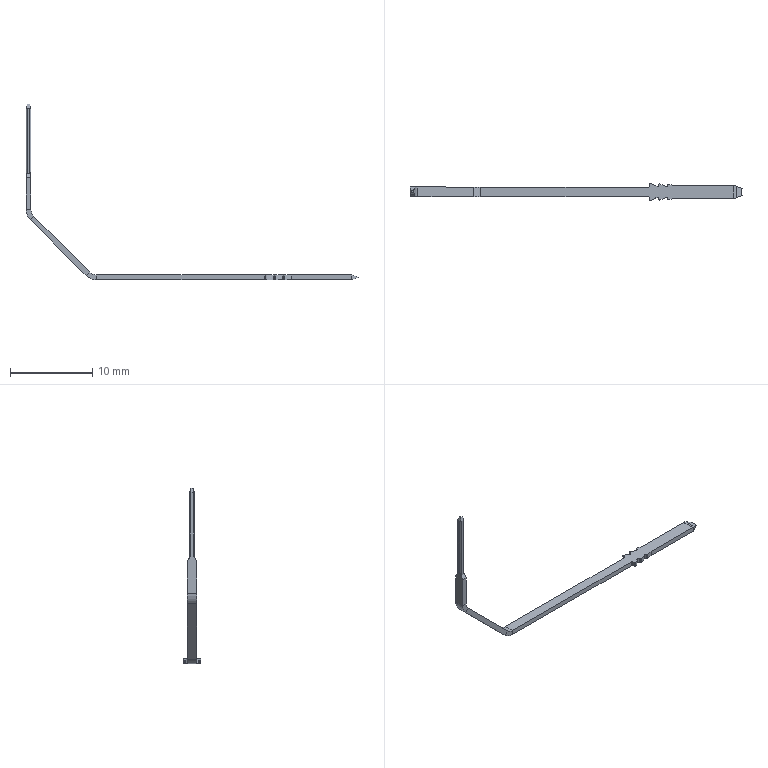Part | NX | features BREP 1 | 1 solid | 77 faces | box 40.3 x 2.1 x 21.3 mm | volume 39.194 mm3 | plane 44 | cylinder 33 | commonest cylinder face diameters 0.3 x12 0.2 x9 0.04 x4 0.025 x2 2 x2 2.4 x2